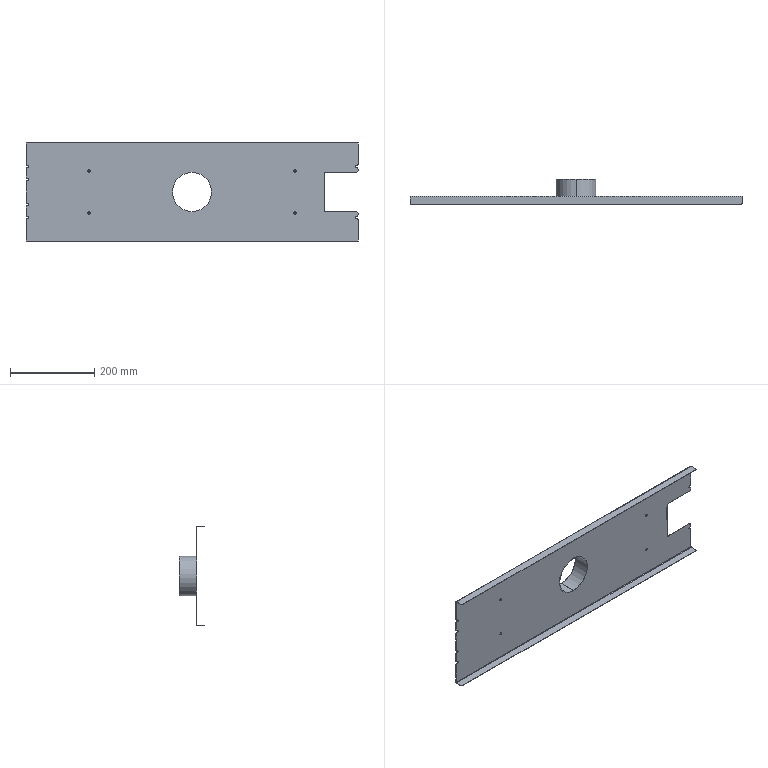Part | SolidWorks | features BaseBody 1 | 1 solid | 73 faces | box 789 x 60 x 237 mm | volume 213070 mm3 | cylinder 40 | plane 33 | commonest cylinder face diameters 6 x18 5.5 x8 5 x6 2 x2 4 x2 93 x2